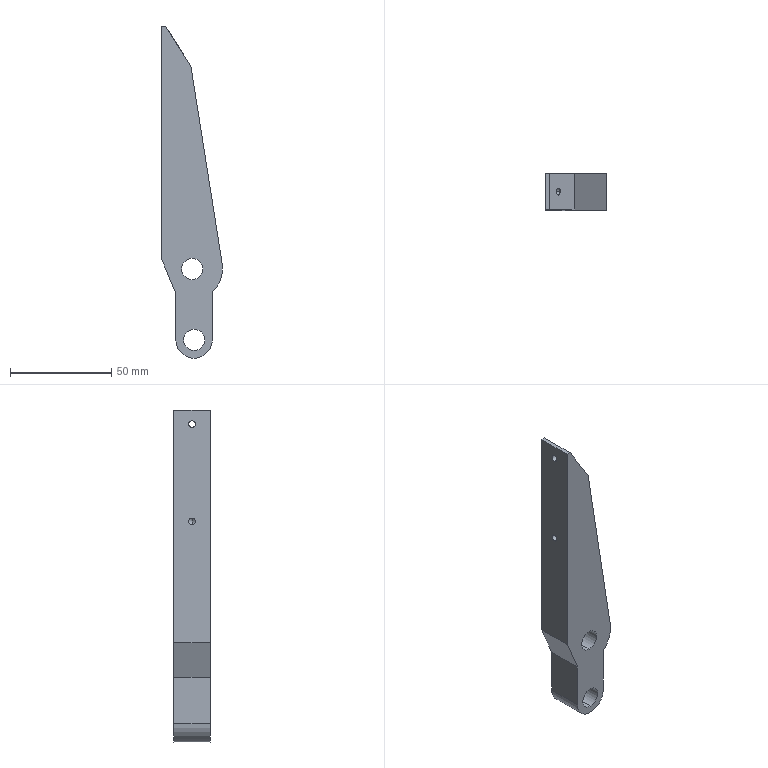Part | SolidWorks | features 3DProfileFeature 1, Extrusion 1, HoleWzd 1 | 1 solid | 22 faces | box 30.153 x 18 x 164 mm | volume 54880 mm3 | cylinder 10 | plane 9 | cone 3 | commonest cylinder face diameters 3.3 x4 10.5 x4 18 x1 30 x1
STEP:
#1=CARTESIAN_POINT('',(7.1,0.,58.35));
#2=VERTEX_POINT('',#1);
#3=CARTESIAN_POINT('',(7.1,0.,61.65));
#4=VERTEX_POINT('',#3);
#5=CARTESIAN_POINT('',(7.1,0.,60.));
#6=DIRECTION('',(-1.,0.,0.));
#7=DIRECTION('',(0.,0.,1.));
#8=AXIS2_PLACEMENT_3D('',#5,#6,#7);
#9=CIRCLE('',#8,1.65);
#10=EDGE_CURVE('',#2,#4,#9,.T.);
#11=ORIENTED_EDGE('',*,*,#10,.F.);
#12=CARTESIAN_POINT('',(0.,0.,58.35));
#13=VERTEX_POINT('',#12);
#14=CARTESIAN_POINT('',(0.,0.,58.35));
#15=DIRECTION('',(-1.,0.,0.));
#16=VECTOR('',#15,1000.);
#17=LINE('',#14,#16);
#18=EDGE_CURVE('',#2,#13,#17,.T.);
#19=ORIENTED_EDGE('',*,*,#18,.T.);
#20=CARTESIAN_POINT('',(0.,0.,61.65));
#21=VERTEX_POINT('',#20);
#22=CARTESIAN_POINT('',(0.,0.,60.));
#23=DIRECTION('',(-1.,0.,0.));
#24=DIRECTION('',(0.,0.,1.));
#25=AXIS2_PLACEMENT_3D('',#22,#23,#24);
#26=CIRCLE('',#25,1.65);
#27=EDGE_CURVE('',#13,#21,#26,.T.);
#28=ORIENTED_EDGE('',*,*,#27,.T.);
#29=CARTESIAN_POINT('',(0.,0.,61.65));
#30=DIRECTION('',(-1.,0.,0.));
#31=VECTOR('',#30,1000.);
#32=LINE('',#29,#31);
#33=EDGE_CURVE('',#4,#21,#32,.T.);
#34=ORIENTED_EDGE('',*,*,#33,.F.);
#35=EDGE_LOOP('',(#11,#19,#28,#34));
#36=FACE_OUTER_BOUND('',#35,.T.);
#37=CARTESIAN_POINT('',(0.,0.,60.));
#38=DIRECTION('',(-1.,0.,0.));
#39=DIRECTION('',(0.,0.,1.));
#40=AXIS2_PLACEMENT_3D('',#37,#38,#39);
#41=CYLINDRICAL_SURFACE('',#40,1.65);
#42=ADVANCED_FACE('',(#36),#41,.F.);
#43=CARTESIAN_POINT('',(8.091,0.,60.));
#44=VERTEX_POINT('',#43);
#45=CARTESIAN_POINT('',(7.1,0.,61.65));
#46=DIRECTION('',(-0.515,0.,0.8572));
#47=VECTOR('',#46,1000.);
#48=LINE('',#45,#47);
#49=EDGE_CURVE('',#44,#4,#48,.T.);
#50=ORIENTED_EDGE('',*,*,#49,.F.);
#51=CARTESIAN_POINT('',(7.1,0.,58.35));
#52=DIRECTION('',(-0.515,0.,-0.8572));
#53=VECTOR('',#52,1000.);
#54=LINE('',#51,#53);
#55=EDGE_CURVE('',#44,#2,#54,.T.);
#56=ORIENTED_EDGE('',*,*,#55,.T.);
#57=ORIENTED_EDGE('',*,*,#10,.T.);
#58=EDGE_LOOP('',(#50,#56,#57));
#59=FACE_OUTER_BOUND('',#58,.T.);
#60=CARTESIAN_POINT('',(7.1,0.,60.));
#61=DIRECTION('',(-1.,0.,0.));
#62=DIRECTION('',(0.,0.,1.));
#63=AXIS2_PLACEMENT_3D('',#60,#61,#62);
#64=CONICAL_SURFACE('',#63,1.65,1.03);
#65=ADVANCED_FACE('',(#59),#64,.F.);
#66=CARTESIAN_POINT('',(7.1,0.,106.35));
#67=VERTEX_POINT('',#66);
#68=CARTESIAN_POINT('',(7.1,-1.173,106.84));
#69=VERTEX_POINT('',#68);
#70=CARTESIAN_POINT('',(7.1,0.,108.));
#71=DIRECTION('',(-1.,0.,0.));
#72=DIRECTION('',(0.,0.,1.));
#73=AXIS2_PLACEMENT_3D('',#70,#71,#72);
#74=CIRCLE('',#73,1.65);
#75=EDGE_CURVE('',#67,#69,#74,.T.);
#76=ORIENTED_EDGE('',*,*,#75,.F.);
#77=CARTESIAN_POINT('',(0.,0.,106.35));
#78=VERTEX_POINT('',#77);
#79=CARTESIAN_POINT('',(0.,0.,106.35));
#80=DIRECTION('',(-1.,0.,0.));
#81=VECTOR('',#80,1000.);
#82=LINE('',#79,#81);
#83=EDGE_CURVE('',#67,#78,#82,.T.);
#84=ORIENTED_EDGE('',*,*,#83,.T.);
#85=CARTESIAN_POINT('',(0.,0.,109.65));
#86=VERTEX_POINT('',#85);
#87=CARTESIAN_POINT('',(0.,0.,108.));
#88=DIRECTION('',(-1.,0.,0.));
#89=DIRECTION('',(0.,0.,1.));
#90=AXIS2_PLACEMENT_3D('',#87,#88,#89);
#91=CIRCLE('',#90,1.65);
#92=EDGE_CURVE('',#78,#86,#91,.T.);
#93=ORIENTED_EDGE('',*,*,#92,.T.);
#94=CARTESIAN_POINT('',(5.344,0.,109.65));
#95=VERTEX_POINT('',#94);
#96=CARTESIAN_POINT('',(0.,0.,109.65));
#97=DIRECTION('',(-1.,0.,0.));
#98=VECTOR('',#97,1000.);
#99=LINE('',#96,#98);
#100=EDGE_CURVE('',#95,#86,#99,.T.);
#101=ORIENTED_EDGE('',*,*,#100,.F.);
#102=CARTESIAN_POINT('',(5.344,0.,109.65));
#103=CARTESIAN_POINT('',(5.344,-1.72,109.65));
#104=CARTESIAN_POINT('',(6.336,-2.382,108.063));
#105=CARTESIAN_POINT('',(7.1,-1.173,106.84));
#106=(BOUNDED_CURVE()B_SPLINE_CURVE(3,(#102,#103,#104,#105),.UNSPECIFIED.,.F.,.F.)B_SPLINE_CURVE_WITH_KNOTS((4,4),(0.,2.35),.UNSPECIFIED.)CURVE()GEOMETRIC_REPRESENTATION_ITEM()RATIONAL_B_SPLINE_CURVE((1.,0.5902,0.5902,1.))REPRESENTATION_ITEM(''));
#107=EDGE_CURVE('',#95,#69,#106,.T.);
#108=ORIENTED_EDGE('',*,*,#107,.T.);
#109=EDGE_LOOP('',(#76,#84,#93,#101,#108));
#110=FACE_OUTER_BOUND('',#109,.T.);
#111=CARTESIAN_POINT('',(0.,0.,108.));
#112=DIRECTION('',(-1.,0.,0.));
#113=DIRECTION('',(0.,0.,1.));
#114=AXIS2_PLACEMENT_3D('',#111,#112,#113);
#115=CYLINDRICAL_SURFACE('',#114,1.65);
#116=ADVANCED_FACE('',(#110),#115,.F.);
#117=CARTESIAN_POINT('',(15.153,-9.,-10.25));
#118=VERTEX_POINT('',#117);
#119=CARTESIAN_POINT('',(15.153,-9.,0.25));
#120=VERTEX_POINT('',#119);
#121=CARTESIAN_POINT('',(15.153,-9.,-5.));
#122=DIRECTION('',(0.,1.,0.));
#123=DIRECTION('',(0.,0.,1.));
#124=AXIS2_PLACEMENT_3D('',#121,#122,#123);
#125=CIRCLE('',#124,5.25);
#126=EDGE_CURVE('',#118,#120,#125,.T.);
#127=ORIENTED_EDGE('',*,*,#126,.F.);
#128=CARTESIAN_POINT('',(15.153,9.,-10.25));
#129=VERTEX_POINT('',#128);
#130=CARTESIAN_POINT('',(15.153,-9.,-10.25));
#131=DIRECTION('',(0.,1.,0.));
#132=VECTOR('',#131,1000.);
#133=LINE('',#130,#132);
#134=EDGE_CURVE('',#118,#129,#133,.T.);
#135=ORIENTED_EDGE('',*,*,#134,.T.);
#136=CARTESIAN_POINT('',(15.153,9.,0.25));
#137=VERTEX_POINT('',#136);
#138=CARTESIAN_POINT('',(15.153,9.,-5.));
#139=DIRECTION('',(0.,1.,0.));
#140=DIRECTION('',(0.,0.,1.));
#141=AXIS2_PLACEMENT_3D('',#138,#139,#140);
#142=CIRCLE('',#141,5.25);
#143=EDGE_CURVE('',#129,#137,#142,.T.);
#144=ORIENTED_EDGE('',*,*,#143,.T.);
#145=CARTESIAN_POINT('',(15.153,-9.,0.25));
#146=DIRECTION('',(0.,1.,0.));
#147=VECTOR('',#146,1000.);
#148=LINE('',#145,#147);
#149=EDGE_CURVE('',#120,#137,#148,.T.);
#150=ORIENTED_EDGE('',*,*,#149,.F.);
#151=EDGE_LOOP('',(#127,#135,#144,#150));
#152=FACE_OUTER_BOUND('',#151,.T.);
#153=CARTESIAN_POINT('',(15.153,-9.,-5.));
#154=DIRECTION('',(0.,1.,0.));
#155=DIRECTION('',(0.,0.,1.));
#156=AXIS2_PLACEMENT_3D('',#153,#154,#155);
#157=CYLINDRICAL_SURFACE('',#156,5.25);
#158=ADVANCED_FACE('',(#152),#157,.F.);
#159=CARTESIAN_POINT('',(16.057,-9.,-45.25));
#160=VERTEX_POINT('',#159);
#161=CARTESIAN_POINT('',(16.057,-9.,-34.75));
#162=VERTEX_POINT('',#161);
#163=CARTESIAN_POINT('',(16.057,-9.,-40.));
#164=DIRECTION('',(0.,1.,0.));
#165=DIRECTION('',(0.,0.,1.));
#166=AXIS2_PLACEMENT_3D('',#163,#164,#165);
#167=CIRCLE('',#166,5.25);
#168=EDGE_CURVE('',#160,#162,#167,.T.);
#169=ORIENTED_EDGE('',*,*,#168,.F.);
#170=CARTESIAN_POINT('',(16.057,9.,-45.25));
#171=VERTEX_POINT('',#170);
#172=CARTESIAN_POINT('',(16.057,-9.,-45.25));
#173=DIRECTION('',(0.,1.,0.));
#174=VECTOR('',#173,1000.);
#175=LINE('',#172,#174);
#176=EDGE_CURVE('',#160,#171,#175,.T.);
#177=ORIENTED_EDGE('',*,*,#176,.T.);
#178=CARTESIAN_POINT('',(16.057,9.,-34.75));
#179=VERTEX_POINT('',#178);
#180=CARTESIAN_POINT('',(16.057,9.,-40.));
#181=DIRECTION('',(0.,1.,0.));
#182=DIRECTION('',(0.,0.,1.));
#183=AXIS2_PLACEMENT_3D('',#180,#181,#182);
#184=CIRCLE('',#183,5.25);
#185=EDGE_CURVE('',#171,#179,#184,.T.);
#186=ORIENTED_EDGE('',*,*,#185,.T.);
#187=CARTESIAN_POINT('',(16.057,-9.,-34.75));
#188=DIRECTION('',(0.,1.,0.));
#189=VECTOR('',#188,1000.);
#190=LINE('',#187,#189);
#191=EDGE_CURVE('',#162,#179,#190,.T.);
#192=ORIENTED_EDGE('',*,*,#191,.F.);
#193=EDGE_LOOP('',(#169,#177,#186,#192));
#194=FACE_OUTER_BOUND('',#193,.T.);
#195=CARTESIAN_POINT('',(16.057,-9.,-40.));
#196=DIRECTION('',(0.,1.,0.));
#197=DIRECTION('',(0.,0.,1.));
#198=AXIS2_PLACEMENT_3D('',#195,#196,#197);
#199=CYLINDRICAL_SURFACE('',#198,5.25);
#200=ADVANCED_FACE('',(#194),#199,.F.);
#201=CARTESIAN_POINT('',(0.,-9.,0.));
#202=VERTEX_POINT('',#201);
#203=CARTESIAN_POINT('',(0.,9.,0.));
#204=VERTEX_POINT('',#203);
#205=CARTESIAN_POINT('',(0.,-9.,0.));
#206=DIRECTION('',(0.,1.,0.));
#207=VECTOR('',#206,1000.);
#208=LINE('',#205,#207);
#209=EDGE_CURVE('',#202,#204,#208,.T.);
#210=ORIENTED_EDGE('',*,*,#209,.T.);
#211=CARTESIAN_POINT('',(7.057,9.,-17.037));
#212=VERTEX_POINT('',#211);
#213=CARTESIAN_POINT('',(0.,9.,0.));
#214=DIRECTION('',(-0.3827,0.,0.9239));
#215=VECTOR('',#214,1000.);
#216=LINE('',#213,#215);
#217=EDGE_CURVE('',#212,#204,#216,.T.);
#218=ORIENTED_EDGE('',*,*,#217,.F.);
#219=CARTESIAN_POINT('',(7.057,-9.,-17.037));
#220=VERTEX_POINT('',#219);
#221=CARTESIAN_POINT('',(7.057,-9.,-17.037));
#222=DIRECTION('',(0.,1.,0.));
#223=VECTOR('',#222,1000.);
#224=LINE('',#221,#223);
#225=EDGE_CURVE('',#220,#212,#224,.T.);
#226=ORIENTED_EDGE('',*,*,#225,.F.);
#227=CARTESIAN_POINT('',(0.,-9.,0.));
#228=DIRECTION('',(-0.3827,0.,0.9239));
#229=VECTOR('',#228,1000.);
#230=LINE('',#227,#229);
#231=EDGE_CURVE('',#220,#202,#230,.T.);
#232=ORIENTED_EDGE('',*,*,#231,.T.);
#233=EDGE_LOOP('',(#210,#218,#226,#232));
#234=FACE_OUTER_BOUND('',#233,.T.);
#235=CARTESIAN_POINT('',(0.,-9.,0.));
#236=DIRECTION('',(-0.9239,0.,-0.3827));
#237=DIRECTION('',(-0.3827,0.,0.9239));
#238=AXIS2_PLACEMENT_3D('',#235,#236,#237);
#239=PLANE('',#238);
#240=ADVANCED_FACE('',(#234),#239,.T.);
#241=ORIENTED_EDGE('',*,*,#225,.T.);
#242=CARTESIAN_POINT('',(7.057,9.,-40.));
#243=VERTEX_POINT('',#242);
#244=CARTESIAN_POINT('',(7.057,9.,-17.037));
#245=DIRECTION('',(0.,0.,1.));
#246=VECTOR('',#245,1000.);
#247=LINE('',#244,#246);
#248=EDGE_CURVE('',#243,#212,#247,.T.);
#249=ORIENTED_EDGE('',*,*,#248,.F.);
#250=CARTESIAN_POINT('',(7.057,-9.,-40.));
#251=VERTEX_POINT('',#250);
#252=CARTESIAN_POINT('',(7.057,-9.,-40.));
#253=DIRECTION('',(0.,1.,0.));
#254=VECTOR('',#253,1000.);
#255=LINE('',#252,#254);
#256=EDGE_CURVE('',#251,#243,#255,.T.);
#257=ORIENTED_EDGE('',*,*,#256,.F.);
#258=CARTESIAN_POINT('',(7.057,-9.,-17.037));
#259=DIRECTION('',(0.,0.,1.));
#260=VECTOR('',#259,1000.);
#261=LINE('',#258,#260);
#262=EDGE_CURVE('',#251,#220,#261,.T.);
#263=ORIENTED_EDGE('',*,*,#262,.T.);
#264=EDGE_LOOP('',(#241,#249,#257,#263));
#265=FACE_OUTER_BOUND('',#264,.T.);
#266=CARTESIAN_POINT('',(7.057,-9.,-17.037));
#267=DIRECTION('',(-1.,0.,0.));
#268=DIRECTION('',(0.,0.,1.));
#269=AXIS2_PLACEMENT_3D('',#266,#267,#268);
#270=PLANE('',#269);
#271=ADVANCED_FACE('',(#265),#270,.T.);
#272=ORIENTED_EDGE('',*,*,#256,.T.);
#273=CARTESIAN_POINT('',(25.057,9.,-40.));
#274=VERTEX_POINT('',#273);
#275=CARTESIAN_POINT('',(16.057,9.,-40.));
#276=DIRECTION('',(0.,1.,0.));
#277=DIRECTION('',(0.,0.,-1.));
#278=AXIS2_PLACEMENT_3D('',#275,#276,#277);
#279=CIRCLE('',#278,9.);
#280=EDGE_CURVE('',#274,#243,#279,.T.);
#281=ORIENTED_EDGE('',*,*,#280,.F.);
#282=CARTESIAN_POINT('',(25.057,-9.,-40.));
#283=VERTEX_POINT('',#282);
#284=CARTESIAN_POINT('',(25.057,-9.,-40.));
#285=DIRECTION('',(0.,1.,0.));
#286=VECTOR('',#285,1000.);
#287=LINE('',#284,#286);
#288=EDGE_CURVE('',#283,#274,#287,.T.);
#289=ORIENTED_EDGE('',*,*,#288,.F.);
#290=CARTESIAN_POINT('',(16.057,-9.,-40.));
#291=DIRECTION('',(0.,1.,0.));
#292=DIRECTION('',(0.,0.,-1.));
#293=AXIS2_PLACEMENT_3D('',#290,#291,#292);
#294=CIRCLE('',#293,9.);
#295=EDGE_CURVE('',#283,#251,#294,.T.);
#296=ORIENTED_EDGE('',*,*,#295,.T.);
#297=EDGE_LOOP('',(#272,#281,#289,#296));
#298=FACE_OUTER_BOUND('',#297,.T.);
#299=CARTESIAN_POINT('',(16.057,-9.,-40.));
#300=DIRECTION('',(0.,1.,0.));
#301=DIRECTION('',(0.,0.,1.));
#302=AXIS2_PLACEMENT_3D('',#299,#300,#301);
#303=CYLINDRICAL_SURFACE('',#302,9.);
#304=ADVANCED_FACE('',(#298),#303,.T.);
#305=ORIENTED_EDGE('',*,*,#288,.T.);
#306=CARTESIAN_POINT('',(25.057,9.,-16.266));
#307=VERTEX_POINT('',#306);
#308=CARTESIAN_POINT('',(25.057,9.,-16.266));
#309=DIRECTION('',(0.,0.,-1.));
#310=VECTOR('',#309,1000.);
#311=LINE('',#308,#310);
#312=EDGE_CURVE('',#307,#274,#311,.T.);
#313=ORIENTED_EDGE('',*,*,#312,.F.);
#314=CARTESIAN_POINT('',(25.057,-9.,-16.266));
#315=VERTEX_POINT('',#314);
#316=CARTESIAN_POINT('',(25.057,-9.,-16.266));
#317=DIRECTION('',(0.,1.,0.));
#318=VECTOR('',#317,1000.);
#319=LINE('',#316,#318);
#320=EDGE_CURVE('',#315,#307,#319,.T.);
#321=ORIENTED_EDGE('',*,*,#320,.F.);
#322=CARTESIAN_POINT('',(25.057,-9.,-16.266));
#323=DIRECTION('',(0.,0.,-1.));
#324=VECTOR('',#323,1000.);
#325=LINE('',#322,#324);
#326=EDGE_CURVE('',#315,#283,#325,.T.);
#327=ORIENTED_EDGE('',*,*,#326,.T.);
#328=EDGE_LOOP('',(#305,#313,#321,#327));
#329=FACE_OUTER_BOUND('',#328,.T.);
#330=CARTESIAN_POINT('',(25.057,-9.,-16.266));
#331=DIRECTION('',(1.,0.,0.));
#332=DIRECTION('',(0.,0.,-1.));
#333=AXIS2_PLACEMENT_3D('',#330,#331,#332);
#334=PLANE('',#333);
#335=ADVANCED_FACE('',(#329),#334,.T.);
#336=ORIENTED_EDGE('',*,*,#320,.T.);
#337=CARTESIAN_POINT('',(30.,9.,-2.863));
#338=VERTEX_POINT('',#337);
#339=CARTESIAN_POINT('',(15.153,9.,-5.));
#340=DIRECTION('',(0.,1.,0.));
#341=DIRECTION('',(0.,0.,1.));
#342=AXIS2_PLACEMENT_3D('',#339,#340,#341);
#343=CIRCLE('',#342,15.);
#344=EDGE_CURVE('',#338,#307,#343,.T.);
#345=ORIENTED_EDGE('',*,*,#344,.F.);
#346=CARTESIAN_POINT('',(30.,-9.,-2.863));
#347=VERTEX_POINT('',#346);
#348=CARTESIAN_POINT('',(30.,-9.,-2.863));
#349=DIRECTION('',(0.,1.,0.));
#350=VECTOR('',#349,1000.);
#351=LINE('',#348,#350);
#352=EDGE_CURVE('',#347,#338,#351,.T.);
#353=ORIENTED_EDGE('',*,*,#352,.F.);
#354=CARTESIAN_POINT('',(15.153,-9.,-5.));
#355=DIRECTION('',(0.,1.,0.));
#356=DIRECTION('',(0.,0.,1.));
#357=AXIS2_PLACEMENT_3D('',#354,#355,#356);
#358=CIRCLE('',#357,15.);
#359=EDGE_CURVE('',#347,#315,#358,.T.);
#360=ORIENTED_EDGE('',*,*,#359,.T.);
#361=EDGE_LOOP('',(#336,#345,#353,#360));
#362=FACE_OUTER_BOUND('',#361,.T.);
#363=CARTESIAN_POINT('',(15.153,-9.,-5.));
#364=DIRECTION('',(0.,1.,0.));
#365=DIRECTION('',(0.,0.,1.));
#366=AXIS2_PLACEMENT_3D('',#363,#364,#365);
#367=CYLINDRICAL_SURFACE('',#366,15.);
#368=ADVANCED_FACE('',(#362),#367,.T.);
#369=ORIENTED_EDGE('',*,*,#352,.T.);
#370=CARTESIAN_POINT('',(14.5,9.,95.));
#371=VERTEX_POINT('',#370);
#372=CARTESIAN_POINT('',(30.,9.,-2.863));
#373=DIRECTION('',(0.1564,0.,-0.9877));
#374=VECTOR('',#373,1000.);
#375=LINE('',#372,#374);
#376=EDGE_CURVE('',#371,#338,#375,.T.);
#377=ORIENTED_EDGE('',*,*,#376,.F.);
#378=CARTESIAN_POINT('',(14.5,-9.,95.));
#379=VERTEX_POINT('',#378);
#380=CARTESIAN_POINT('',(14.5,-9.,95.));
#381=DIRECTION('',(0.,1.,0.));
#382=VECTOR('',#381,1000.);
#383=LINE('',#380,#382);
#384=EDGE_CURVE('',#379,#371,#383,.T.);
#385=ORIENTED_EDGE('',*,*,#384,.F.);
#386=CARTESIAN_POINT('',(30.,-9.,-2.863));
#387=DIRECTION('',(0.1564,0.,-0.9877));
#388=VECTOR('',#387,1000.);
#389=LINE('',#386,#388);
#390=EDGE_CURVE('',#379,#347,#389,.T.);
#391=ORIENTED_EDGE('',*,*,#390,.T.);
#392=EDGE_LOOP('',(#369,#377,#385,#391));
#393=FACE_OUTER_BOUND('',#392,.T.);
#394=CARTESIAN_POINT('',(30.,-9.,-2.863));
#395=DIRECTION('',(0.9877,0.,0.1564));
#396=DIRECTION('',(0.1564,0.,-0.9877));
#397=AXIS2_PLACEMENT_3D('',#394,#395,#396);
#398=PLANE('',#397);
#399=ADVANCED_FACE('',(#393),#398,.T.);
#400=CARTESIAN_POINT('',(7.1,1.173,106.84));
#401=VERTEX_POINT('',#400);
#402=CARTESIAN_POINT('',(7.1,1.173,106.84));
#403=CARTESIAN_POINT('',(6.336,2.382,108.063));
#404=CARTESIAN_POINT('',(5.344,1.72,109.65));
#405=CARTESIAN_POINT('',(5.344,0.,109.65));
#406=(BOUNDED_CURVE()B_SPLINE_CURVE(3,(#402,#403,#404,#405),.UNSPECIFIED.,.F.,.F.)B_SPLINE_CURVE_WITH_KNOTS((4,4),(3.933,6.283),.UNSPECIFIED.)CURVE()GEOMETRIC_REPRESENTATION_ITEM()RATIONAL_B_SPLINE_CURVE((1.,0.5902,0.5902,1.))REPRESENTATION_ITEM(''));
#407=EDGE_CURVE('',#401,#95,#406,.T.);
#408=ORIENTED_EDGE('',*,*,#407,.F.);
#409=CARTESIAN_POINT('',(7.1,-1.173,106.84));
#410=CARTESIAN_POINT('',(7.147,-0.9893,106.765));
#411=CARTESIAN_POINT('',(7.184,-0.7996,106.705));
#412=CARTESIAN_POINT('',(7.236,-0.407,106.622));
#413=CARTESIAN_POINT('',(7.25,-0.2015,106.6));
#414=CARTESIAN_POINT('',(7.25,0.2014,106.6));
#415=CARTESIAN_POINT('',(7.237,0.4011,106.621));
#416=CARTESIAN_POINT('',(7.185,0.7975,106.704));
#417=CARTESIAN_POINT('',(7.147,0.9891,106.765));
#418=CARTESIAN_POINT('',(7.1,1.173,106.84));
#419=B_SPLINE_CURVE_WITH_KNOTS('',3,(#409,#410,#411,#412,#413,#414,#415,#416,#417,#418),.UNSPECIFIED.,.F.,.F.,(4,2,2,2,4),(0.00000086,0.0006069,0.001213,0.001819,0.002425),.UNSPECIFIED.);
#420=EDGE_CURVE('',#69,#401,#419,.T.);
#421=ORIENTED_EDGE('',*,*,#420,.F.);
#422=ORIENTED_EDGE('',*,*,#107,.F.);
#423=EDGE_LOOP('',(#408,#421,#422));
#424=FACE_BOUND('',#423,.T.);
#425=ORIENTED_EDGE('',*,*,#384,.T.);
#426=CARTESIAN_POINT('',(2.,9.,115.));
#427=VERTEX_POINT('',#426);
#428=CARTESIAN_POINT('',(14.5,9.,95.));
#429=DIRECTION('',(0.53,0.,-0.848));
#430=VECTOR('',#429,1000.);
#431=LINE('',#428,#430);
#432=EDGE_CURVE('',#427,#371,#431,.T.);
#433=ORIENTED_EDGE('',*,*,#432,.F.);
#434=CARTESIAN_POINT('',(2.,-9.,115.));
#435=VERTEX_POINT('',#434);
#436=CARTESIAN_POINT('',(2.,-9.,115.));
#437=DIRECTION('',(0.,1.,0.));
#438=VECTOR('',#437,1000.);
#439=LINE('',#436,#438);
#440=EDGE_CURVE('',#435,#427,#439,.T.);
#441=ORIENTED_EDGE('',*,*,#440,.F.);
#442=CARTESIAN_POINT('',(14.5,-9.,95.));
#443=DIRECTION('',(0.53,0.,-0.848));
#444=VECTOR('',#443,1000.);
#445=LINE('',#442,#444);
#446=EDGE_CURVE('',#435,#379,#445,.T.);
#447=ORIENTED_EDGE('',*,*,#446,.T.);
#448=EDGE_LOOP('',(#425,#433,#441,#447));
#449=FACE_OUTER_BOUND('',#448,.T.);
#450=CARTESIAN_POINT('',(14.5,-9.,95.));
#451=DIRECTION('',(0.848,0.,0.53));
#452=DIRECTION('',(0.53,0.,-0.848));
#453=AXIS2_PLACEMENT_3D('',#450,#451,#452);
#454=PLANE('',#453);
#455=ADVANCED_FACE('',(#424,#449),#454,.T.);
#456=ORIENTED_EDGE('',*,*,#440,.T.);
#457=CARTESIAN_POINT('',(0.,9.,115.));
#458=VERTEX_POINT('',#457);
#459=CARTESIAN_POINT('',(0.,9.,115.));
#460=DIRECTION('',(1.,0.,0.));
#461=VECTOR('',#460,1000.);
#462=LINE('',#459,#461);
#463=EDGE_CURVE('',#458,#427,#462,.T.);
#464=ORIENTED_EDGE('',*,*,#463,.F.);
#465=CARTESIAN_POINT('',(0.,-9.,115.));
#466=VERTEX_POINT('',#465);
#467=CARTESIAN_POINT('',(0.,-9.,115.));
#468=DIRECTION('',(0.,1.,0.));
#469=VECTOR('',#468,1000.);
#470=LINE('',#467,#469);
#471=EDGE_CURVE('',#466,#458,#470,.T.);
#472=ORIENTED_EDGE('',*,*,#471,.F.);
#473=CARTESIAN_POINT('',(0.,-9.,115.));
#474=DIRECTION('',(1.,0.,0.));
#475=VECTOR('',#474,1000.);
#476=LINE('',#473,#475);
#477=EDGE_CURVE('',#466,#435,#476,.T.);
#478=ORIENTED_EDGE('',*,*,#477,.T.);
#479=EDGE_LOOP('',(#456,#464,#472,#478));
#480=FACE_OUTER_BOUND('',#479,.T.);
#481=CARTESIAN_POINT('',(0.,-9.,115.));
#482=DIRECTION('',(0.,0.,1.));
#483=DIRECTION('',(1.,0.,0.));
#484=AXIS2_PLACEMENT_3D('',#481,#482,#483);
#485=PLANE('',#484);
#486=ADVANCED_FACE('',(#480),#485,.T.);
#487=CARTESIAN_POINT('',(0.,0.,60.));
#488=DIRECTION('',(-1.,0.,0.));
#489=DIRECTION('',(0.,0.,1.));
#490=AXIS2_PLACEMENT_3D('',#487,#488,#489);
#491=CIRCLE('',#490,1.65);
#492=EDGE_CURVE('',#21,#13,#491,.T.);
#493=ORIENTED_EDGE('',*,*,#492,.F.);
#494=ORIENTED_EDGE('',*,*,#27,.F.);
#495=EDGE_LOOP('',(#493,#494));
#496=FACE_BOUND('',#495,.T.);
#497=CARTESIAN_POINT('',(0.,0.,108.));
#498=DIRECTION('',(-1.,0.,0.));
#499=DIRECTION('',(0.,0.,1.));
#500=AXIS2_PLACEMENT_3D('',#497,#498,#499);
#501=CIRCLE('',#500,1.65);
#502=EDGE_CURVE('',#86,#78,#501,.T.);
#503=ORIENTED_EDGE('',*,*,#502,.F.);
#504=ORIENTED_EDGE('',*,*,#92,.F.);
#505=EDGE_LOOP('',(#503,#504));
#506=FACE_BOUND('',#505,.T.);
#507=ORIENTED_EDGE('',*,*,#471,.T.);
#508=CARTESIAN_POINT('',(0.,9.,0.));
#509=DIRECTION('',(0.,0.,1.));
#510=VECTOR('',#509,1000.);
#511=LINE('',#508,#510);
#512=EDGE_CURVE('',#204,#458,#511,.T.);
#513=ORIENTED_EDGE('',*,*,#512,.F.);
#514=ORIENTED_EDGE('',*,*,#209,.F.);
#515=CARTESIAN_POINT('',(0.,-9.,0.));
#516=DIRECTION('',(0.,0.,1.));
#517=VECTOR('',#516,1000.);
#518=LINE('',#515,#517);
#519=EDGE_CURVE('',#202,#466,#518,.T.);
#520=ORIENTED_EDGE('',*,*,#519,.T.);
#521=EDGE_LOOP('',(#507,#513,#514,#520));
#522=FACE_OUTER_BOUND('',#521,.T.);
#523=CARTESIAN_POINT('',(0.,-9.,0.));
#524=DIRECTION('',(-1.,0.,0.));
#525=DIRECTION('',(0.,0.,1.));
#526=AXIS2_PLACEMENT_3D('',#523,#524,#525);
#527=PLANE('',#526);
#528=ADVANCED_FACE('',(#496,#506,#522),#527,.T.);
#529=CARTESIAN_POINT('',(15.153,-9.,-5.));
#530=DIRECTION('',(0.,1.,0.));
#531=DIRECTION('',(0.,0.,1.));
#532=AXIS2_PLACEMENT_3D('',#529,#530,#531);
#533=CIRCLE('',#532,5.25);
#534=EDGE_CURVE('',#120,#118,#533,.T.);
#535=ORIENTED_EDGE('',*,*,#534,.T.);
#536=ORIENTED_EDGE('',*,*,#126,.T.);
#537=EDGE_LOOP('',(#535,#536));
#538=FACE_BOUND('',#537,.T.);
#539=CARTESIAN_POINT('',(16.057,-9.,-40.));
#540=DIRECTION('',(0.,1.,0.));
#541=DIRECTION('',(0.,0.,1.));
#542=AXIS2_PLACEMENT_3D('',#539,#540,#541);
#543=CIRCLE('',#542,5.25);
#544=EDGE_CURVE('',#162,#160,#543,.T.);
#545=ORIENTED_EDGE('',*,*,#544,.T.);
#546=ORIENTED_EDGE('',*,*,#168,.T.);
#547=EDGE_LOOP('',(#545,#546));
#548=FACE_BOUND('',#547,.T.);
#549=ORIENTED_EDGE('',*,*,#231,.F.);
#550=ORIENTED_EDGE('',*,*,#262,.F.);
#551=ORIENTED_EDGE('',*,*,#295,.F.);
#552=ORIENTED_EDGE('',*,*,#326,.F.);
#553=ORIENTED_EDGE('',*,*,#359,.F.);
#554=ORIENTED_EDGE('',*,*,#390,.F.);
#555=ORIENTED_EDGE('',*,*,#446,.F.);
#556=ORIENTED_EDGE('',*,*,#477,.F.);
#557=ORIENTED_EDGE('',*,*,#519,.F.);
#558=EDGE_LOOP('',(#549,#550,#551,#552,#553,#554,#555,#556,#557));
#559=FACE_OUTER_BOUND('',#558,.T.);
#560=CARTESIAN_POINT('',(16.057,-9.,-40.));
#561=DIRECTION('',(0.,-1.,0.));
#562=DIRECTION('',(0.,0.,-1.));
#563=AXIS2_PLACEMENT_3D('',#560,#561,#562);
#564=PLANE('',#563);
#565=ADVANCED_FACE('',(#538,#548,#559),#564,.T.);
#566=ORIENTED_EDGE('',*,*,#176,.F.);
#567=ORIENTED_EDGE('',*,*,#544,.F.);
#568=ORIENTED_EDGE('',*,*,#191,.T.);
#569=CARTESIAN_POINT('',(16.057,9.,-40.));
#570=DIRECTION('',(0.,1.,0.));
#571=DIRECTION('',(0.,0.,1.));
#572=AXIS2_PLACEMENT_3D('',#569,#570,#571);
#573=CIRCLE('',#572,5.25);
#574=EDGE_CURVE('',#179,#171,#573,.T.);
#575=ORIENTED_EDGE('',*,*,#574,.T.);
#576=EDGE_LOOP('',(#566,#567,#568,#575));
#577=FACE_OUTER_BOUND('',#576,.T.);
#578=CARTESIAN_POINT('',(16.057,-9.,-40.));
#579=DIRECTION('',(0.,1.,0.));
#580=DIRECTION('',(0.,0.,1.));
#581=AXIS2_PLACEMENT_3D('',#578,#579,#580);
#582=CYLINDRICAL_SURFACE('',#581,5.25);
#583=ADVANCED_FACE('',(#577),#582,.F.);
#584=ORIENTED_EDGE('',*,*,#134,.F.);
#585=ORIENTED_EDGE('',*,*,#534,.F.);
#586=ORIENTED_EDGE('',*,*,#149,.T.);
#587=CARTESIAN_POINT('',(15.153,9.,-5.));
#588=DIRECTION('',(0.,1.,0.));
#589=DIRECTION('',(0.,0.,1.));
#590=AXIS2_PLACEMENT_3D('',#587,#588,#589);
#591=CIRCLE('',#590,5.25);
#592=EDGE_CURVE('',#137,#129,#591,.T.);
#593=ORIENTED_EDGE('',*,*,#592,.T.);
#594=EDGE_LOOP('',(#584,#585,#586,#593));
#595=FACE_OUTER_BOUND('',#594,.T.);
#596=CARTESIAN_POINT('',(15.153,-9.,-5.));
#597=DIRECTION('',(0.,1.,0.));
#598=DIRECTION('',(0.,0.,1.));
#599=AXIS2_PLACEMENT_3D('',#596,#597,#598);
#600=CYLINDRICAL_SURFACE('',#599,5.25);
#601=ADVANCED_FACE('',(#595),#600,.F.);
#602=ORIENTED_EDGE('',*,*,#574,.F.);
#603=ORIENTED_EDGE('',*,*,#185,.F.);
#604=EDGE_LOOP('',(#602,#603));
#605=FACE_BOUND('',#604,.T.);
#606=ORIENTED_EDGE('',*,*,#217,.T.);
#607=ORIENTED_EDGE('',*,*,#512,.T.);
#608=ORIENTED_EDGE('',*,*,#463,.T.);
#609=ORIENTED_EDGE('',*,*,#432,.T.);
#610=ORIENTED_EDGE('',*,*,#376,.T.);
#611=ORIENTED_EDGE('',*,*,#344,.T.);
#612=ORIENTED_EDGE('',*,*,#312,.T.);
#613=ORIENTED_EDGE('',*,*,#280,.T.);
#614=ORIENTED_EDGE('',*,*,#248,.T.);
#615=EDGE_LOOP('',(#606,#607,#608,#609,#610,#611,#612,#613,#614));
#616=FACE_OUTER_BOUND('',#615,.T.);
#617=ORIENTED_EDGE('',*,*,#592,.F.);
#618=ORIENTED_EDGE('',*,*,#143,.F.);
#619=EDGE_LOOP('',(#617,#618));
#620=FACE_BOUND('',#619,.T.);
#621=CARTESIAN_POINT('',(16.057,9.,-40.));
#622=DIRECTION('',(0.,-1.,0.));
#623=DIRECTION('',(0.,0.,-1.));
#624=AXIS2_PLACEMENT_3D('',#621,#622,#623);
#625=PLANE('',#624);
#626=ADVANCED_FACE('',(#605,#616,#620),#625,.F.);
#627=ORIENTED_EDGE('',*,*,#420,.T.);
#628=CARTESIAN_POINT('',(7.1,0.,108.));
#629=DIRECTION('',(-1.,0.,0.));
#630=DIRECTION('',(0.,0.,1.));
#631=AXIS2_PLACEMENT_3D('',#628,#629,#630);
#632=CIRCLE('',#631,1.65);
#633=EDGE_CURVE('',#401,#67,#632,.T.);
#634=ORIENTED_EDGE('',*,*,#633,.T.);
#635=ORIENTED_EDGE('',*,*,#75,.T.);
#636=EDGE_LOOP('',(#627,#634,#635));
#637=FACE_OUTER_BOUND('',#636,.T.);
#638=CARTESIAN_POINT('',(7.1,0.,108.));
#639=DIRECTION('',(-1.,0.,0.));
#640=DIRECTION('',(0.,0.,1.));
#641=AXIS2_PLACEMENT_3D('',#638,#639,#640);
#642=CONICAL_SURFACE('',#641,1.65,1.03);
#643=ADVANCED_FACE('',(#637),#642,.F.);
#644=ORIENTED_EDGE('',*,*,#83,.F.);
#645=ORIENTED_EDGE('',*,*,#633,.F.);
#646=ORIENTED_EDGE('',*,*,#407,.T.);
#647=ORIENTED_EDGE('',*,*,#100,.T.);
#648=ORIENTED_EDGE('',*,*,#502,.T.);
#649=EDGE_LOOP('',(#644,#645,#646,#647,#648));
#650=FACE_OUTER_BOUND('',#649,.T.);
#651=CARTESIAN_POINT('',(0.,0.,108.));
#652=DIRECTION('',(-1.,0.,0.));
#653=DIRECTION('',(0.,0.,1.));
#654=AXIS2_PLACEMENT_3D('',#651,#652,#653);
#655=CYLINDRICAL_SURFACE('',#654,1.65);
#656=ADVANCED_FACE('',(#650),#655,.F.);
#657=ORIENTED_EDGE('',*,*,#55,.F.);
#658=ORIENTED_EDGE('',*,*,#49,.T.);
#659=CARTESIAN_POINT('',(7.1,0.,60.));
#660=DIRECTION('',(-1.,0.,0.));
#661=DIRECTION('',(0.,0.,1.));
#662=AXIS2_PLACEMENT_3D('',#659,#660,#661);
#663=CIRCLE('',#662,1.65);
#664=EDGE_CURVE('',#4,#2,#663,.T.);
#665=ORIENTED_EDGE('',*,*,#664,.T.);
#666=EDGE_LOOP('',(#657,#658,#665));
#667=FACE_OUTER_BOUND('',#666,.T.);
#668=CARTESIAN_POINT('',(7.1,0.,60.));
#669=DIRECTION('',(-1.,0.,0.));
#670=DIRECTION('',(0.,0.,1.));
#671=AXIS2_PLACEMENT_3D('',#668,#669,#670);
#672=CONICAL_SURFACE('',#671,1.65,1.03);
#673=ADVANCED_FACE('',(#667),#672,.F.);
#674=ORIENTED_EDGE('',*,*,#18,.F.);
#675=ORIENTED_EDGE('',*,*,#664,.F.);
#676=ORIENTED_EDGE('',*,*,#33,.T.);
#677=ORIENTED_EDGE('',*,*,#492,.T.);
#678=EDGE_LOOP('',(#674,#675,#676,#677));
#679=FACE_OUTER_BOUND('',#678,.T.);
#680=CARTESIAN_POINT('',(0.,0.,60.));
#681=DIRECTION('',(-1.,0.,0.));
#682=DIRECTION('',(0.,0.,1.));
#683=AXIS2_PLACEMENT_3D('',#680,#681,#682);
#684=CYLINDRICAL_SURFACE('',#683,1.65);
#685=ADVANCED_FACE('',(#679),#684,.F.);
#686=CLOSED_SHELL('',(#42,#65,#116,#158,#200,#240,#271,#304,#335,#368,#399,#455,#486,#528,#565,#583,#601,#626,#643,#656,#673,#685));
#687=MANIFOLD_SOLID_BREP('',#686);
#688=CARTESIAN_POINT('',(0.,0.,0.));
#689=DIRECTION('',(0.,0.,1.));
#690=DIRECTION('',(1.,0.,0.));
#691=AXIS2_PLACEMENT_3D('',#688,#689,#690);
#692=(LENGTH_UNIT()NAMED_UNIT(*)SI_UNIT(.MILLI.,.METRE.));
#693=UNCERTAINTY_MEASURE_WITH_UNIT(LENGTH_MEASURE(0.00001),#692,'','');
#694=(NAMED_UNIT(*)PLANE_ANGLE_UNIT()SI_UNIT($,.RADIAN.));
#695=(NAMED_UNIT(*)SI_UNIT($,.STERADIAN.)SOLID_ANGLE_UNIT());
#696=(GEOMETRIC_REPRESENTATION_CONTEXT(3)GLOBAL_UNCERTAINTY_ASSIGNED_CONTEXT((#693))GLOBAL_UNIT_ASSIGNED_CONTEXT((#692,#694,#695))REPRESENTATION_CONTEXT('',''));
#697=ADVANCED_BREP_SHAPE_REPRESENTATION('',(#687,#691),#696);